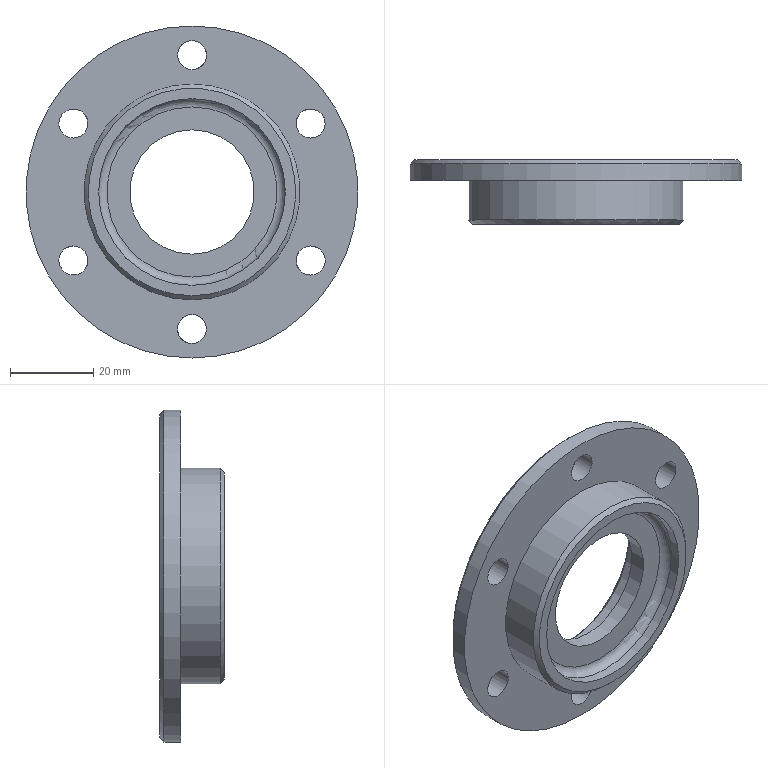Part | NX | features DATUM_CSYS 3, SKETCH 2, EXTRUDE 1, SWP104 1 | 1 solid | 20 faces | box 80 x 15.5 x 80 mm | volume 27346 mm3 | cylinder 11 | plane 5 | cone 3 | torus 1 | commonest cylinder face diameters 7 x6 30 x1 40 x1 45 x1 52 x1 80 x1
STEP:
#1=CARTESIAN_POINT('',(0.,0.,-22.5));
#2=VERTEX_POINT('',#1);
#3=CARTESIAN_POINT('',(0.,0.,0.));
#4=DIRECTION('',(0.,-1.,0.));
#5=DIRECTION('',(0.,0.,-1.));
#6=AXIS2_PLACEMENT_3D('',#3,#4,#5);
#7=CIRCLE('',#6,22.5);
#8=EDGE_CURVE('',#2,#2,#7,.T.);
#9=ORIENTED_EDGE('',*,*,#8,.F.);
#10=EDGE_LOOP('',(#9));
#11=FACE_BOUND('',#10,.T.);
#12=CARTESIAN_POINT('',(0.,0.,-25.));
#13=VERTEX_POINT('',#12);
#14=CARTESIAN_POINT('',(0.,0.,0.));
#15=DIRECTION('',(0.,-1.,0.));
#16=DIRECTION('',(0.,0.,-1.));
#17=AXIS2_PLACEMENT_3D('',#14,#15,#16);
#18=CIRCLE('',#17,25.);
#19=EDGE_CURVE('',#13,#13,#18,.T.);
#20=ORIENTED_EDGE('',*,*,#19,.T.);
#21=EDGE_LOOP('',(#20));
#22=FACE_BOUND('',#21,.T.);
#23=CARTESIAN_POINT('',(0.,0.,25.));
#24=DIRECTION('',(0.,1.,0.));
#25=DIRECTION('',(0.,0.,1.));
#26=AXIS2_PLACEMENT_3D('',#23,#24,#25);
#27=PLANE('',#26);
#28=ADVANCED_FACE('',(#11,#22),#27,.F.);
#29=CARTESIAN_POINT('',(0.,2.5,-22.5));
#30=VERTEX_POINT('',#29);
#31=CARTESIAN_POINT('',(0.,2.5,0.));
#32=DIRECTION('',(0.,-1.,0.));
#33=DIRECTION('',(0.,0.,-1.));
#34=AXIS2_PLACEMENT_3D('',#31,#32,#33);
#35=CIRCLE('',#34,22.5);
#36=EDGE_CURVE('',#30,#30,#35,.T.);
#37=ORIENTED_EDGE('',*,*,#36,.F.);
#38=EDGE_LOOP('',(#37));
#39=FACE_BOUND('',#38,.T.);
#40=ORIENTED_EDGE('',*,*,#8,.T.);
#41=EDGE_LOOP('',(#40));
#42=FACE_BOUND('',#41,.T.);
#43=CARTESIAN_POINT('',(0.,0.,0.));
#44=DIRECTION('',(0.,-1.,0.));
#45=DIRECTION('',(0.,0.,-1.));
#46=AXIS2_PLACEMENT_3D('',#43,#44,#45);
#47=CYLINDRICAL_SURFACE('',#46,22.5);
#48=ADVANCED_FACE('',(#39,#42),#47,.F.);
#49=CARTESIAN_POINT('',(0.,4.5,-20.5));
#50=VERTEX_POINT('',#49);
#51=CARTESIAN_POINT('',(0.,4.5,0.));
#52=DIRECTION('',(0.,-1.,0.));
#53=DIRECTION('',(0.,0.,-1.));
#54=AXIS2_PLACEMENT_3D('',#51,#52,#53);
#55=CIRCLE('',#54,20.5);
#56=EDGE_CURVE('',#50,#50,#55,.T.);
#57=ORIENTED_EDGE('',*,*,#56,.F.);
#58=EDGE_LOOP('',(#57));
#59=FACE_BOUND('',#58,.T.);
#60=ORIENTED_EDGE('',*,*,#36,.T.);
#61=EDGE_LOOP('',(#60));
#62=FACE_BOUND('',#61,.T.);
#63=CARTESIAN_POINT('',(0.,2.5,0.));
#64=DIRECTION('',(0.,-1.,0.));
#65=DIRECTION('',(0.,0.,-1.));
#66=AXIS2_PLACEMENT_3D('',#63,#64,#65);
#67=TOROIDAL_SURFACE('',#66,20.5,2.);
#68=ADVANCED_FACE('',(#59,#62),#67,.F.);
#69=CARTESIAN_POINT('',(0.,4.5,-15.));
#70=VERTEX_POINT('',#69);
#71=CARTESIAN_POINT('',(0.,4.5,0.));
#72=DIRECTION('',(0.,-1.,0.));
#73=DIRECTION('',(0.,0.,-1.));
#74=AXIS2_PLACEMENT_3D('',#71,#72,#73);
#75=CIRCLE('',#74,15.);
#76=EDGE_CURVE('',#70,#70,#75,.T.);
#77=ORIENTED_EDGE('',*,*,#76,.F.);
#78=EDGE_LOOP('',(#77));
#79=FACE_BOUND('',#78,.T.);
#80=ORIENTED_EDGE('',*,*,#56,.T.);
#81=EDGE_LOOP('',(#80));
#82=FACE_BOUND('',#81,.T.);
#83=CARTESIAN_POINT('',(0.,4.5,20.5));
#84=DIRECTION('',(0.,1.,0.));
#85=DIRECTION('',(0.,0.,1.));
#86=AXIS2_PLACEMENT_3D('',#83,#84,#85);
#87=PLANE('',#86);
#88=ADVANCED_FACE('',(#79,#82),#87,.F.);
#89=CARTESIAN_POINT('',(0.,8.5,-15.));
#90=VERTEX_POINT('',#89);
#91=CARTESIAN_POINT('',(0.,8.5,0.));
#92=DIRECTION('',(0.,-1.,0.));
#93=DIRECTION('',(0.,0.,-1.));
#94=AXIS2_PLACEMENT_3D('',#91,#92,#93);
#95=CIRCLE('',#94,15.);
#96=EDGE_CURVE('',#90,#90,#95,.T.);
#97=ORIENTED_EDGE('',*,*,#96,.F.);
#98=EDGE_LOOP('',(#97));
#99=FACE_BOUND('',#98,.T.);
#100=ORIENTED_EDGE('',*,*,#76,.T.);
#101=EDGE_LOOP('',(#100));
#102=FACE_BOUND('',#101,.T.);
#103=CARTESIAN_POINT('',(0.,0.,0.));
#104=DIRECTION('',(0.,-1.,0.));
#105=DIRECTION('',(0.,0.,-1.));
#106=AXIS2_PLACEMENT_3D('',#103,#104,#105);
#107=CYLINDRICAL_SURFACE('',#106,15.);
#108=ADVANCED_FACE('',(#99,#102),#107,.F.);
#109=CARTESIAN_POINT('',(0.,8.5,-20.));
#110=VERTEX_POINT('',#109);
#111=CARTESIAN_POINT('',(0.,8.5,0.));
#112=DIRECTION('',(0.,-1.,0.));
#113=DIRECTION('',(0.,0.,-1.));
#114=AXIS2_PLACEMENT_3D('',#111,#112,#113);
#115=CIRCLE('',#114,20.);
#116=EDGE_CURVE('',#110,#110,#115,.T.);
#117=ORIENTED_EDGE('',*,*,#116,.F.);
#118=EDGE_LOOP('',(#117));
#119=FACE_BOUND('',#118,.T.);
#120=ORIENTED_EDGE('',*,*,#96,.T.);
#121=EDGE_LOOP('',(#120));
#122=FACE_BOUND('',#121,.T.);
#123=CARTESIAN_POINT('',(0.,8.5,15.));
#124=DIRECTION('',(0.,-1.,0.));
#125=DIRECTION('',(0.,0.,-1.));
#126=AXIS2_PLACEMENT_3D('',#123,#124,#125);
#127=PLANE('',#126);
#128=ADVANCED_FACE('',(#119,#122),#127,.F.);
#129=CARTESIAN_POINT('',(0.,14.5,-20.));
#130=VERTEX_POINT('',#129);
#131=CARTESIAN_POINT('',(0.,14.5,0.));
#132=DIRECTION('',(0.,-1.,0.));
#133=DIRECTION('',(0.,0.,-1.));
#134=AXIS2_PLACEMENT_3D('',#131,#132,#133);
#135=CIRCLE('',#134,20.);
#136=EDGE_CURVE('',#130,#130,#135,.T.);
#137=ORIENTED_EDGE('',*,*,#136,.F.);
#138=EDGE_LOOP('',(#137));
#139=FACE_BOUND('',#138,.T.);
#140=ORIENTED_EDGE('',*,*,#116,.T.);
#141=EDGE_LOOP('',(#140));
#142=FACE_BOUND('',#141,.T.);
#143=CARTESIAN_POINT('',(0.,0.,0.));
#144=DIRECTION('',(0.,-1.,0.));
#145=DIRECTION('',(0.,0.,-1.));
#146=AXIS2_PLACEMENT_3D('',#143,#144,#145);
#147=CYLINDRICAL_SURFACE('',#146,20.);
#148=ADVANCED_FACE('',(#139,#142),#147,.F.);
#149=CARTESIAN_POINT('',(0.,15.5,-21.));
#150=VERTEX_POINT('',#149);
#151=CARTESIAN_POINT('',(0.,15.5,0.));
#152=DIRECTION('',(0.,-1.,0.));
#153=DIRECTION('',(0.,0.,-1.));
#154=AXIS2_PLACEMENT_3D('',#151,#152,#153);
#155=CIRCLE('',#154,21.);
#156=EDGE_CURVE('',#150,#150,#155,.T.);
#157=ORIENTED_EDGE('',*,*,#156,.F.);
#158=EDGE_LOOP('',(#157));
#159=FACE_BOUND('',#158,.T.);
#160=ORIENTED_EDGE('',*,*,#136,.T.);
#161=EDGE_LOOP('',(#160));
#162=FACE_BOUND('',#161,.T.);
#163=CARTESIAN_POINT('',(0.,14.5,0.));
#164=DIRECTION('',(0.,1.,0.));
#165=DIRECTION('',(0.,0.,1.));
#166=AXIS2_PLACEMENT_3D('',#163,#164,#165);
#167=CONICAL_SURFACE('',#166,20.,0.7854);
#168=ADVANCED_FACE('',(#159,#162),#167,.F.);
#169=CARTESIAN_POINT('',(28.579,15.5,13.));
#170=VERTEX_POINT('',#169);
#171=CARTESIAN_POINT('',(28.579,15.5,16.5));
#172=DIRECTION('',(0.,-1.,0.));
#173=DIRECTION('',(0.,0.,-1.));
#174=AXIS2_PLACEMENT_3D('',#171,#172,#173);
#175=CIRCLE('',#174,3.5);
#176=EDGE_CURVE('',#170,#170,#175,.T.);
#177=ORIENTED_EDGE('',*,*,#176,.T.);
#178=EDGE_LOOP('',(#177));
#179=FACE_BOUND('',#178,.T.);
#180=CARTESIAN_POINT('',(0.,15.5,29.5));
#181=VERTEX_POINT('',#180);
#182=CARTESIAN_POINT('',(0.,15.5,33.));
#183=DIRECTION('',(0.,-1.,0.));
#184=DIRECTION('',(0.,0.,-1.));
#185=AXIS2_PLACEMENT_3D('',#182,#183,#184);
#186=CIRCLE('',#185,3.5);
#187=EDGE_CURVE('',#181,#181,#186,.T.);
#188=ORIENTED_EDGE('',*,*,#187,.T.);
#189=EDGE_LOOP('',(#188));
#190=FACE_BOUND('',#189,.T.);
#191=CARTESIAN_POINT('',(-28.579,15.5,13.));
#192=VERTEX_POINT('',#191);
#193=CARTESIAN_POINT('',(-28.579,15.5,16.5));
#194=DIRECTION('',(0.,-1.,0.));
#195=DIRECTION('',(0.,0.,-1.));
#196=AXIS2_PLACEMENT_3D('',#193,#194,#195);
#197=CIRCLE('',#196,3.5);
#198=EDGE_CURVE('',#192,#192,#197,.T.);
#199=ORIENTED_EDGE('',*,*,#198,.T.);
#200=EDGE_LOOP('',(#199));
#201=FACE_BOUND('',#200,.T.);
#202=CARTESIAN_POINT('',(-28.579,15.5,-20.));
#203=VERTEX_POINT('',#202);
#204=CARTESIAN_POINT('',(-28.579,15.5,-16.5));
#205=DIRECTION('',(0.,-1.,0.));
#206=DIRECTION('',(0.,0.,-1.));
#207=AXIS2_PLACEMENT_3D('',#204,#205,#206);
#208=CIRCLE('',#207,3.5);
#209=EDGE_CURVE('',#203,#203,#208,.T.);
#210=ORIENTED_EDGE('',*,*,#209,.T.);
#211=EDGE_LOOP('',(#210));
#212=FACE_BOUND('',#211,.T.);
#213=CARTESIAN_POINT('',(0.,15.5,-36.5));
#214=VERTEX_POINT('',#213);
#215=CARTESIAN_POINT('',(0.,15.5,-33.));
#216=DIRECTION('',(0.,-1.,0.));
#217=DIRECTION('',(0.,0.,-1.));
#218=AXIS2_PLACEMENT_3D('',#215,#216,#217);
#219=CIRCLE('',#218,3.5);
#220=EDGE_CURVE('',#214,#214,#219,.T.);
#221=ORIENTED_EDGE('',*,*,#220,.T.);
#222=EDGE_LOOP('',(#221));
#223=FACE_BOUND('',#222,.T.);
#224=CARTESIAN_POINT('',(28.579,15.5,-20.));
#225=VERTEX_POINT('',#224);
#226=CARTESIAN_POINT('',(28.579,15.5,-16.5));
#227=DIRECTION('',(0.,-1.,0.));
#228=DIRECTION('',(0.,0.,-1.));
#229=AXIS2_PLACEMENT_3D('',#226,#227,#228);
#230=CIRCLE('',#229,3.5);
#231=EDGE_CURVE('',#225,#225,#230,.T.);
#232=ORIENTED_EDGE('',*,*,#231,.T.);
#233=EDGE_LOOP('',(#232));
#234=FACE_BOUND('',#233,.T.);
#235=CARTESIAN_POINT('',(0.,15.5,-39.));
#236=VERTEX_POINT('',#235);
#237=CARTESIAN_POINT('',(0.,15.5,0.));
#238=DIRECTION('',(0.,-1.,0.));
#239=DIRECTION('',(0.,0.,-1.));
#240=AXIS2_PLACEMENT_3D('',#237,#238,#239);
#241=CIRCLE('',#240,39.);
#242=EDGE_CURVE('',#236,#236,#241,.T.);
#243=ORIENTED_EDGE('',*,*,#242,.F.);
#244=EDGE_LOOP('',(#243));
#245=FACE_BOUND('',#244,.T.);
#246=ORIENTED_EDGE('',*,*,#156,.T.);
#247=EDGE_LOOP('',(#246));
#248=FACE_BOUND('',#247,.T.);
#249=CARTESIAN_POINT('',(0.,15.5,21.));
#250=DIRECTION('',(0.,-1.,0.));
#251=DIRECTION('',(0.,0.,-1.));
#252=AXIS2_PLACEMENT_3D('',#249,#250,#251);
#253=PLANE('',#252);
#254=ADVANCED_FACE('',(#179,#190,#201,#212,#223,#234,#245,#248),#253,.F.);
#255=CARTESIAN_POINT('',(0.,14.5,-40.));
#256=VERTEX_POINT('',#255);
#257=CARTESIAN_POINT('',(0.,14.5,0.));
#258=DIRECTION('',(0.,-1.,0.));
#259=DIRECTION('',(0.,0.,-1.));
#260=AXIS2_PLACEMENT_3D('',#257,#258,#259);
#261=CIRCLE('',#260,40.);
#262=EDGE_CURVE('',#256,#256,#261,.T.);
#263=ORIENTED_EDGE('',*,*,#262,.F.);
#264=EDGE_LOOP('',(#263));
#265=FACE_BOUND('',#264,.T.);
#266=ORIENTED_EDGE('',*,*,#242,.T.);
#267=EDGE_LOOP('',(#266));
#268=FACE_BOUND('',#267,.T.);
#269=CARTESIAN_POINT('',(0.,15.5,0.));
#270=DIRECTION('',(0.,-1.,0.));
#271=DIRECTION('',(0.,0.,-1.));
#272=AXIS2_PLACEMENT_3D('',#269,#270,#271);
#273=CONICAL_SURFACE('',#272,39.,0.7854);
#274=ADVANCED_FACE('',(#265,#268),#273,.T.);
#275=CARTESIAN_POINT('',(0.,10.5,-40.));
#276=VERTEX_POINT('',#275);
#277=CARTESIAN_POINT('',(0.,10.5,0.));
#278=DIRECTION('',(0.,-1.,0.));
#279=DIRECTION('',(0.,0.,-1.));
#280=AXIS2_PLACEMENT_3D('',#277,#278,#279);
#281=CIRCLE('',#280,40.);
#282=EDGE_CURVE('',#276,#276,#281,.T.);
#283=ORIENTED_EDGE('',*,*,#282,.F.);
#284=EDGE_LOOP('',(#283));
#285=FACE_BOUND('',#284,.T.);
#286=ORIENTED_EDGE('',*,*,#262,.T.);
#287=EDGE_LOOP('',(#286));
#288=FACE_BOUND('',#287,.T.);
#289=CARTESIAN_POINT('',(0.,0.,0.));
#290=DIRECTION('',(0.,-1.,0.));
#291=DIRECTION('',(0.,0.,-1.));
#292=AXIS2_PLACEMENT_3D('',#289,#290,#291);
#293=CYLINDRICAL_SURFACE('',#292,40.);
#294=ADVANCED_FACE('',(#285,#288),#293,.T.);
#295=CARTESIAN_POINT('',(30.329,10.5,13.469));
#296=VERTEX_POINT('',#295);
#297=CARTESIAN_POINT('',(28.579,10.5,16.5));
#298=DIRECTION('',(0.,-1.,0.));
#299=DIRECTION('',(0.5,0.,-0.866));
#300=AXIS2_PLACEMENT_3D('',#297,#298,#299);
#301=CIRCLE('',#300,3.5);
#302=EDGE_CURVE('',#296,#296,#301,.T.);
#303=ORIENTED_EDGE('',*,*,#302,.F.);
#304=EDGE_LOOP('',(#303));
#305=FACE_BOUND('',#304,.T.);
#306=CARTESIAN_POINT('',(3.5,10.5,33.));
#307=VERTEX_POINT('',#306);
#308=CARTESIAN_POINT('',(0.,10.5,33.));
#309=DIRECTION('',(0.,-1.,0.));
#310=DIRECTION('',(1.,0.,0.));
#311=AXIS2_PLACEMENT_3D('',#308,#309,#310);
#312=CIRCLE('',#311,3.5);
#313=EDGE_CURVE('',#307,#307,#312,.T.);
#314=ORIENTED_EDGE('',*,*,#313,.F.);
#315=EDGE_LOOP('',(#314));
#316=FACE_BOUND('',#315,.T.);
#317=CARTESIAN_POINT('',(-26.829,10.5,19.531));
#318=VERTEX_POINT('',#317);
#319=CARTESIAN_POINT('',(-28.579,10.5,16.5));
#320=DIRECTION('',(0.,-1.,0.));
#321=DIRECTION('',(0.5,0.,0.866));
#322=AXIS2_PLACEMENT_3D('',#319,#320,#321);
#323=CIRCLE('',#322,3.5);
#324=EDGE_CURVE('',#318,#318,#323,.T.);
#325=ORIENTED_EDGE('',*,*,#324,.F.);
#326=EDGE_LOOP('',(#325));
#327=FACE_BOUND('',#326,.T.);
#328=CARTESIAN_POINT('',(-30.329,10.5,-13.469));
#329=VERTEX_POINT('',#328);
#330=CARTESIAN_POINT('',(-28.579,10.5,-16.5));
#331=DIRECTION('',(0.,-1.,0.));
#332=DIRECTION('',(-0.5,0.,0.866));
#333=AXIS2_PLACEMENT_3D('',#330,#331,#332);
#334=CIRCLE('',#333,3.5);
#335=EDGE_CURVE('',#329,#329,#334,.T.);
#336=ORIENTED_EDGE('',*,*,#335,.F.);
#337=EDGE_LOOP('',(#336));
#338=FACE_BOUND('',#337,.T.);
#339=CARTESIAN_POINT('',(-3.5,10.5,-33.));
#340=VERTEX_POINT('',#339);
#341=CARTESIAN_POINT('',(0.,10.5,-33.));
#342=DIRECTION('',(0.,-1.,0.));
#343=DIRECTION('',(-1.,0.,0.));
#344=AXIS2_PLACEMENT_3D('',#341,#342,#343);
#345=CIRCLE('',#344,3.5);
#346=EDGE_CURVE('',#340,#340,#345,.T.);
#347=ORIENTED_EDGE('',*,*,#346,.F.);
#348=EDGE_LOOP('',(#347));
#349=FACE_BOUND('',#348,.T.);
#350=CARTESIAN_POINT('',(26.829,10.5,-19.531));
#351=VERTEX_POINT('',#350);
#352=CARTESIAN_POINT('',(28.579,10.5,-16.5));
#353=DIRECTION('',(0.,-1.,0.));
#354=DIRECTION('',(-0.5,0.,-0.866));
#355=AXIS2_PLACEMENT_3D('',#352,#353,#354);
#356=CIRCLE('',#355,3.5);
#357=EDGE_CURVE('',#351,#351,#356,.T.);
#358=ORIENTED_EDGE('',*,*,#357,.F.);
#359=EDGE_LOOP('',(#358));
#360=FACE_BOUND('',#359,.T.);
#361=CARTESIAN_POINT('',(0.,10.5,-26.));
#362=VERTEX_POINT('',#361);
#363=CARTESIAN_POINT('',(0.,10.5,0.));
#364=DIRECTION('',(0.,-1.,0.));
#365=DIRECTION('',(0.,0.,-1.));
#366=AXIS2_PLACEMENT_3D('',#363,#364,#365);
#367=CIRCLE('',#366,26.);
#368=EDGE_CURVE('',#362,#362,#367,.T.);
#369=ORIENTED_EDGE('',*,*,#368,.F.);
#370=EDGE_LOOP('',(#369));
#371=FACE_BOUND('',#370,.T.);
#372=ORIENTED_EDGE('',*,*,#282,.T.);
#373=EDGE_LOOP('',(#372));
#374=FACE_BOUND('',#373,.T.);
#375=CARTESIAN_POINT('',(0.,10.5,40.));
#376=DIRECTION('',(0.,1.,0.));
#377=DIRECTION('',(0.,0.,1.));
#378=AXIS2_PLACEMENT_3D('',#375,#376,#377);
#379=PLANE('',#378);
#380=ADVANCED_FACE('',(#305,#316,#327,#338,#349,#360,#371,#374),#379,.F.);
#381=CARTESIAN_POINT('',(0.,1.,-26.));
#382=VERTEX_POINT('',#381);
#383=CARTESIAN_POINT('',(0.,1.,0.));
#384=DIRECTION('',(0.,-1.,0.));
#385=DIRECTION('',(0.,0.,-1.));
#386=AXIS2_PLACEMENT_3D('',#383,#384,#385);
#387=CIRCLE('',#386,26.);
#388=EDGE_CURVE('',#382,#382,#387,.T.);
#389=ORIENTED_EDGE('',*,*,#388,.F.);
#390=EDGE_LOOP('',(#389));
#391=FACE_BOUND('',#390,.T.);
#392=ORIENTED_EDGE('',*,*,#368,.T.);
#393=EDGE_LOOP('',(#392));
#394=FACE_BOUND('',#393,.T.);
#395=CARTESIAN_POINT('',(0.,0.,0.));
#396=DIRECTION('',(0.,-1.,0.));
#397=DIRECTION('',(0.,0.,-1.));
#398=AXIS2_PLACEMENT_3D('',#395,#396,#397);
#399=CYLINDRICAL_SURFACE('',#398,26.);
#400=ADVANCED_FACE('',(#391,#394),#399,.T.);
#401=ORIENTED_EDGE('',*,*,#19,.F.);
#402=EDGE_LOOP('',(#401));
#403=FACE_BOUND('',#402,.T.);
#404=ORIENTED_EDGE('',*,*,#388,.T.);
#405=EDGE_LOOP('',(#404));
#406=FACE_BOUND('',#405,.T.);
#407=CARTESIAN_POINT('',(0.,1.,0.));
#408=DIRECTION('',(0.,1.,0.));
#409=DIRECTION('',(0.,0.,1.));
#410=AXIS2_PLACEMENT_3D('',#407,#408,#409);
#411=CONICAL_SURFACE('',#410,26.,0.7854);
#412=ADVANCED_FACE('',(#403,#406),#411,.T.);
#413=ORIENTED_EDGE('',*,*,#357,.T.);
#414=EDGE_LOOP('',(#413));
#415=FACE_BOUND('',#414,.T.);
#416=ORIENTED_EDGE('',*,*,#231,.F.);
#417=EDGE_LOOP('',(#416));
#418=FACE_BOUND('',#417,.T.);
#419=CARTESIAN_POINT('',(28.579,41.5,-16.5));
#420=DIRECTION('',(0.,-1.,0.));
#421=DIRECTION('',(0.,0.,-1.));
#422=AXIS2_PLACEMENT_3D('',#419,#420,#421);
#423=CYLINDRICAL_SURFACE('',#422,3.5);
#424=ADVANCED_FACE('',(#415,#418),#423,.F.);
#425=ORIENTED_EDGE('',*,*,#346,.T.);
#426=EDGE_LOOP('',(#425));
#427=FACE_BOUND('',#426,.T.);
#428=ORIENTED_EDGE('',*,*,#220,.F.);
#429=EDGE_LOOP('',(#428));
#430=FACE_BOUND('',#429,.T.);
#431=CARTESIAN_POINT('',(0.,41.5,-33.));
#432=DIRECTION('',(0.,-1.,0.));
#433=DIRECTION('',(0.,0.,-1.));
#434=AXIS2_PLACEMENT_3D('',#431,#432,#433);
#435=CYLINDRICAL_SURFACE('',#434,3.5);
#436=ADVANCED_FACE('',(#427,#430),#435,.F.);
#437=ORIENTED_EDGE('',*,*,#335,.T.);
#438=EDGE_LOOP('',(#437));
#439=FACE_BOUND('',#438,.T.);
#440=ORIENTED_EDGE('',*,*,#209,.F.);
#441=EDGE_LOOP('',(#440));
#442=FACE_BOUND('',#441,.T.);
#443=CARTESIAN_POINT('',(-28.579,41.5,-16.5));
#444=DIRECTION('',(0.,-1.,0.));
#445=DIRECTION('',(0.,0.,-1.));
#446=AXIS2_PLACEMENT_3D('',#443,#444,#445);
#447=CYLINDRICAL_SURFACE('',#446,3.5);
#448=ADVANCED_FACE('',(#439,#442),#447,.F.);
#449=ORIENTED_EDGE('',*,*,#324,.T.);
#450=EDGE_LOOP('',(#449));
#451=FACE_BOUND('',#450,.T.);
#452=ORIENTED_EDGE('',*,*,#198,.F.);
#453=EDGE_LOOP('',(#452));
#454=FACE_BOUND('',#453,.T.);
#455=CARTESIAN_POINT('',(-28.579,41.5,16.5));
#456=DIRECTION('',(0.,-1.,0.));
#457=DIRECTION('',(0.,0.,-1.));
#458=AXIS2_PLACEMENT_3D('',#455,#456,#457);
#459=CYLINDRICAL_SURFACE('',#458,3.5);
#460=ADVANCED_FACE('',(#451,#454),#459,.F.);
#461=ORIENTED_EDGE('',*,*,#313,.T.);
#462=EDGE_LOOP('',(#461));
#463=FACE_BOUND('',#462,.T.);
#464=ORIENTED_EDGE('',*,*,#187,.F.);
#465=EDGE_LOOP('',(#464));
#466=FACE_BOUND('',#465,.T.);
#467=CARTESIAN_POINT('',(0.,41.5,33.));
#468=DIRECTION('',(0.,-1.,0.));
#469=DIRECTION('',(0.,0.,-1.));
#470=AXIS2_PLACEMENT_3D('',#467,#468,#469);
#471=CYLINDRICAL_SURFACE('',#470,3.5);
#472=ADVANCED_FACE('',(#463,#466),#471,.F.);
#473=ORIENTED_EDGE('',*,*,#302,.T.);
#474=EDGE_LOOP('',(#473));
#475=FACE_BOUND('',#474,.T.);
#476=ORIENTED_EDGE('',*,*,#176,.F.);
#477=EDGE_LOOP('',(#476));
#478=FACE_BOUND('',#477,.T.);
#479=CARTESIAN_POINT('',(28.579,41.5,16.5));
#480=DIRECTION('',(0.,-1.,0.));
#481=DIRECTION('',(0.,0.,-1.));
#482=AXIS2_PLACEMENT_3D('',#479,#480,#481);
#483=CYLINDRICAL_SURFACE('',#482,3.5);
#484=ADVANCED_FACE('',(#475,#478),#483,.F.);
#485=CLOSED_SHELL('',(#28,#48,#68,#88,#108,#128,#148,#168,#254,#274,#294,#380,#400,#412,#424,#436,#448,#460,#472,#484));
#486=MANIFOLD_SOLID_BREP('',#485);
#487=(LENGTH_UNIT()NAMED_UNIT(*)SI_UNIT(.MILLI.,.METRE.));
#488=UNCERTAINTY_MEASURE_WITH_UNIT(LENGTH_MEASURE(0.00001),#487,'','');
#489=(NAMED_UNIT(*)PLANE_ANGLE_UNIT()SI_UNIT($,.RADIAN.));
#490=(NAMED_UNIT(*)SI_UNIT($,.STERADIAN.)SOLID_ANGLE_UNIT());
#491=(GEOMETRIC_REPRESENTATION_CONTEXT(3)GLOBAL_UNCERTAINTY_ASSIGNED_CONTEXT((#488))GLOBAL_UNIT_ASSIGNED_CONTEXT((#487,#489,#490))REPRESENTATION_CONTEXT('',''));
#492=ADVANCED_BREP_SHAPE_REPRESENTATION('',(#486),#491);